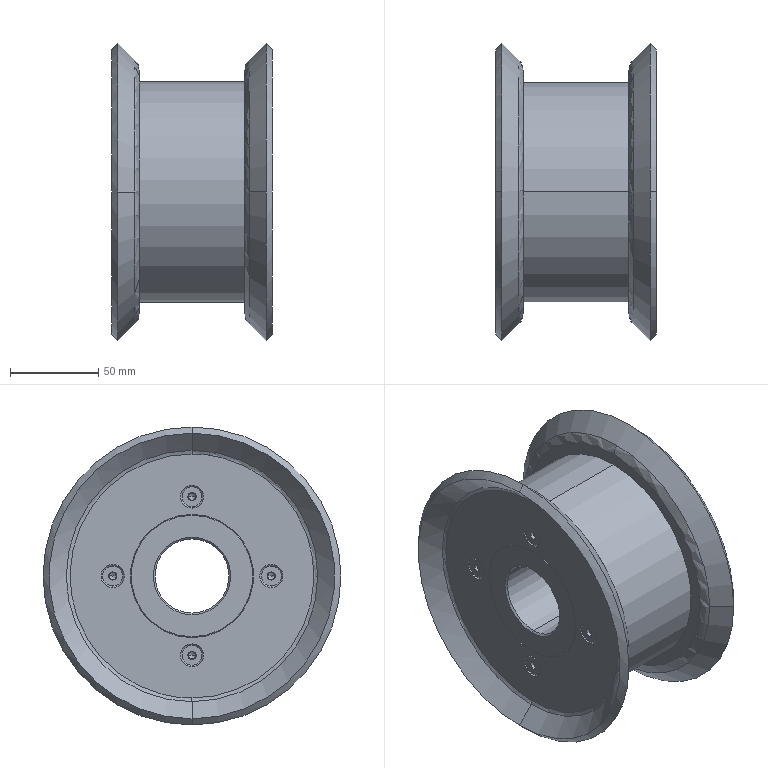Part | SolidWorks | 10 solids | 704 faces | box 91.113 x 169.042 x 169.042 mm | volume 833344 mm3 | cylinder 280 | cone 174 | plane 130 | spline 120 | commonest cylinder face diameters 6 x200 5 x16 6.6 x16 11.34 x16 13 x16 70 x8